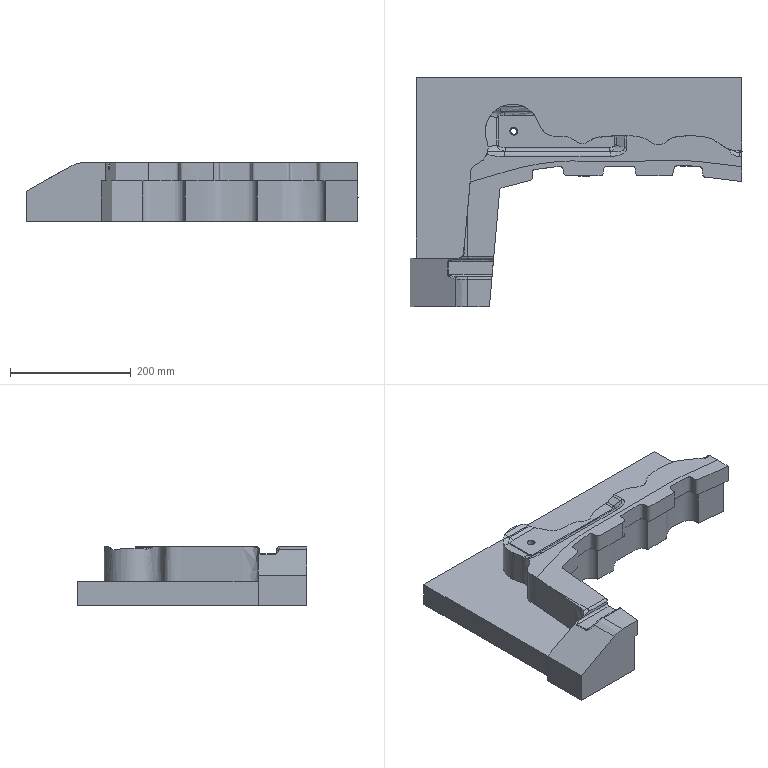Part | NX | features solid 2 | 1 solid | 74 faces | box 550.001 x 380 x 97 mm | volume 6391201 mm3 | spline 70 | plane 3 | cylinder 1 | commonest cylinder face diameters 13 x1